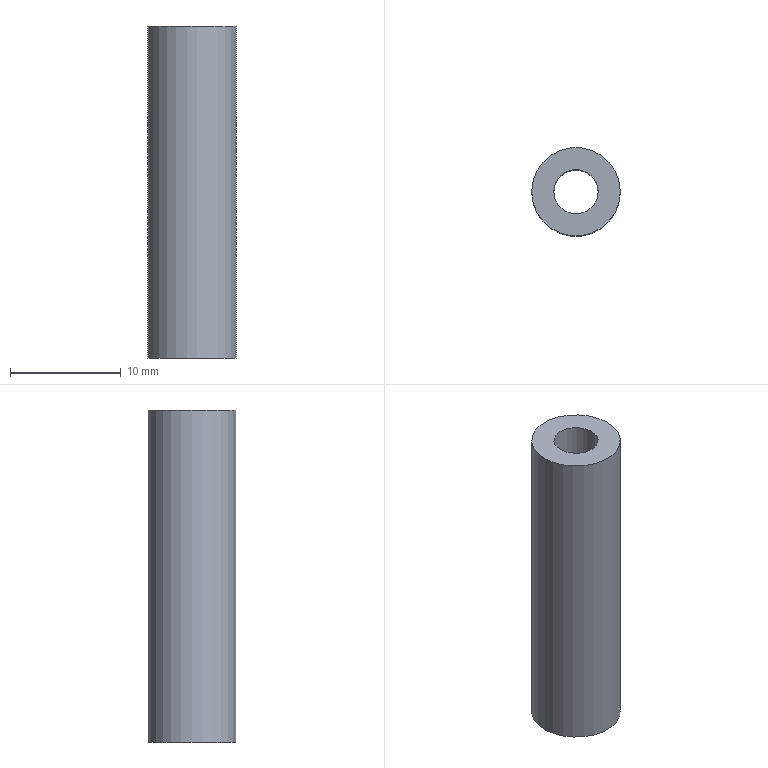Part | STEP file | gslz 2016.10.28-10_id2042_x_t | 1 solid | 4 faces | box 8 x 8 x 30 mm | volume 1131 mm3 | cylinder 2 | plane 2 | commonest cylinder face diameters 4 x1 8 x1
STEP:
#1=CARTESIAN_POINT('',(0.,0.,0.));
#2=DIRECTION('',(0.,0.,1.));
#3=DIRECTION('',(1.,0.,0.));
#4=AXIS2_PLACEMENT_3D('',#1,#2,#3);
#5=CARTESIAN_POINT('',(-541.,163.,53.));
#6=VERTEX_POINT('',#5);
#7=CARTESIAN_POINT('',(-545.,163.,53.));
#8=DIRECTION('',(0.,0.,1.));
#9=DIRECTION('',(1.,0.,0.));
#10=AXIS2_PLACEMENT_3D('',#7,#8,#9);
#11=CIRCLE('',#10,4.);
#12=CARTESIAN_POINT('',(-545.,163.,53.));
#13=DIRECTION('',(0.,0.,-1.));
#14=DIRECTION('',(1.,0.,0.));
#15=AXIS2_PLACEMENT_3D('',#12,#13,#14);
#16=CYLINDRICAL_SURFACE('',#15,4.);
#17=CARTESIAN_POINT('',(6.283,0.));
#18=DIRECTION('',(-1.,0.));
#19=VECTOR('',#18,1.);
#20=LINE('',#17,#19);
#21=(GEOMETRIC_REPRESENTATION_CONTEXT(2)PARAMETRIC_REPRESENTATION_CONTEXT()REPRESENTATION_CONTEXT('',''));
#22=DEFINITIONAL_REPRESENTATION('',(#20),#21);
#23=PCURVE('',#16,#22);
#24=CARTESIAN_POINT('',(-545.,163.,53.));
#25=DIRECTION('',(0.,0.,1.));
#26=DIRECTION('',(-1.,0.,0.));
#27=AXIS2_PLACEMENT_3D('',#24,#25,#26);
#28=PLANE('',#27);
#29=CARTESIAN_POINT('',(0.,0.));
#30=DIRECTION('',(-1.,0.));
#31=AXIS2_PLACEMENT_2D('',#29,#30);
#32=CIRCLE('',#31,4.);
#33=(GEOMETRIC_REPRESENTATION_CONTEXT(2)PARAMETRIC_REPRESENTATION_CONTEXT()REPRESENTATION_CONTEXT('',''));
#34=DEFINITIONAL_REPRESENTATION('',(#32),#33);
#35=PCURVE('',#28,#34);
#36=SURFACE_CURVE('',#11,(#23,#35),.PCURVE_S1.);
#37=EDGE_CURVE('',#6,#6,#36,.T.);
#38=ORIENTED_EDGE('',*,*,#37,.F.);
#39=CARTESIAN_POINT('',(-541.,163.,23.));
#40=VERTEX_POINT('',#39);
#41=CARTESIAN_POINT('',(-541.,163.,53.));
#42=CARTESIAN_POINT('',(-541.,163.,23.));
#43=B_SPLINE_CURVE_WITH_KNOTS('',1,(#41,#42),.UNSPECIFIED.,.F.,.F.,(2,2),(0.,30.),.PIECEWISE_BEZIER_KNOTS.);
#44=CARTESIAN_POINT('',(6.283,0.));
#45=DIRECTION('',(0.,1.));
#46=VECTOR('',#45,1.);
#47=LINE('',#44,#46);
#48=(GEOMETRIC_REPRESENTATION_CONTEXT(2)PARAMETRIC_REPRESENTATION_CONTEXT()REPRESENTATION_CONTEXT('',''));
#49=DEFINITIONAL_REPRESENTATION('',(#47),#48);
#50=PCURVE('',#16,#49);
#51=CARTESIAN_POINT('',(0.,0.));
#52=DIRECTION('',(0.,1.));
#53=VECTOR('',#52,1.);
#54=LINE('',#51,#53);
#55=(GEOMETRIC_REPRESENTATION_CONTEXT(2)PARAMETRIC_REPRESENTATION_CONTEXT()REPRESENTATION_CONTEXT('',''));
#56=DEFINITIONAL_REPRESENTATION('',(#54),#55);
#57=PCURVE('',#16,#56);
#58=SEAM_CURVE('',#43,(#50,#57),.PCURVE_S1.);
#59=EDGE_CURVE('',#6,#40,#58,.T.);
#60=ORIENTED_EDGE('',*,*,#59,.T.);
#61=CARTESIAN_POINT('',(-545.,163.,23.));
#62=DIRECTION('',(0.,0.,1.));
#63=DIRECTION('',(1.,0.,0.));
#64=AXIS2_PLACEMENT_3D('',#61,#62,#63);
#65=CIRCLE('',#64,4.);
#66=CARTESIAN_POINT('',(6.283,30.));
#67=DIRECTION('',(-1.,0.));
#68=VECTOR('',#67,1.);
#69=LINE('',#66,#68);
#70=(GEOMETRIC_REPRESENTATION_CONTEXT(2)PARAMETRIC_REPRESENTATION_CONTEXT()REPRESENTATION_CONTEXT('',''));
#71=DEFINITIONAL_REPRESENTATION('',(#69),#70);
#72=PCURVE('',#16,#71);
#73=CARTESIAN_POINT('',(-545.,163.,23.));
#74=DIRECTION('',(0.,0.,1.));
#75=DIRECTION('',(-1.,0.,0.));
#76=AXIS2_PLACEMENT_3D('',#73,#74,#75);
#77=PLANE('',#76);
#78=CARTESIAN_POINT('',(0.,0.));
#79=DIRECTION('',(-1.,0.));
#80=AXIS2_PLACEMENT_2D('',#78,#79);
#81=CIRCLE('',#80,4.);
#82=(GEOMETRIC_REPRESENTATION_CONTEXT(2)PARAMETRIC_REPRESENTATION_CONTEXT()REPRESENTATION_CONTEXT('',''));
#83=DEFINITIONAL_REPRESENTATION('',(#81),#82);
#84=PCURVE('',#77,#83);
#85=SURFACE_CURVE('',#65,(#72,#84),.PCURVE_S1.);
#86=EDGE_CURVE('',#40,#40,#85,.T.);
#87=ORIENTED_EDGE('',*,*,#86,.T.);
#88=ORIENTED_EDGE('',*,*,#59,.F.);
#89=EDGE_LOOP('',(#38,#60,#87,#88));
#90=FACE_BOUND('',#89,.T.);
#91=ADVANCED_FACE('',(#90),#16,.T.);
#92=CARTESIAN_POINT('',(-543.,163.,53.));
#93=VERTEX_POINT('',#92);
#94=CARTESIAN_POINT('',(-545.,163.,53.));
#95=DIRECTION('',(0.,0.,1.));
#96=DIRECTION('',(1.,0.,0.));
#97=AXIS2_PLACEMENT_3D('',#94,#95,#96);
#98=CIRCLE('',#97,2.);
#99=CARTESIAN_POINT('',(0.,0.));
#100=DIRECTION('',(-1.,0.));
#101=AXIS2_PLACEMENT_2D('',#99,#100);
#102=CIRCLE('',#101,2.);
#103=(GEOMETRIC_REPRESENTATION_CONTEXT(2)PARAMETRIC_REPRESENTATION_CONTEXT()REPRESENTATION_CONTEXT('',''));
#104=DEFINITIONAL_REPRESENTATION('',(#102),#103);
#105=PCURVE('',#28,#104);
#106=CARTESIAN_POINT('',(-545.,163.,-7.));
#107=DIRECTION('',(0.,0.,1.));
#108=DIRECTION('',(-1.,0.,0.));
#109=AXIS2_PLACEMENT_3D('',#106,#107,#108);
#110=CYLINDRICAL_SURFACE('',#109,2.);
#111=CARTESIAN_POINT('',(3.142,60.));
#112=DIRECTION('',(1.,0.));
#113=VECTOR('',#112,1.);
#114=LINE('',#111,#113);
#115=(GEOMETRIC_REPRESENTATION_CONTEXT(2)PARAMETRIC_REPRESENTATION_CONTEXT()REPRESENTATION_CONTEXT('',''));
#116=DEFINITIONAL_REPRESENTATION('',(#114),#115);
#117=PCURVE('',#110,#116);
#118=SURFACE_CURVE('',#98,(#105,#117),.PCURVE_S1.);
#119=EDGE_CURVE('',#93,#93,#118,.T.);
#120=ORIENTED_EDGE('',*,*,#119,.F.);
#121=EDGE_LOOP('',(#120));
#122=FACE_BOUND('',#121,.T.);
#123=ORIENTED_EDGE('',*,*,#37,.T.);
#124=EDGE_LOOP('',(#123));
#125=FACE_BOUND('',#124,.T.);
#126=ADVANCED_FACE('',(#122,#125),#28,.T.);
#127=CARTESIAN_POINT('',(-543.,163.,23.));
#128=VERTEX_POINT('',#127);
#129=CARTESIAN_POINT('',(-545.,163.,23.));
#130=DIRECTION('',(0.,0.,1.));
#131=DIRECTION('',(1.,0.,0.));
#132=AXIS2_PLACEMENT_3D('',#129,#130,#131);
#133=CIRCLE('',#132,2.);
#134=CARTESIAN_POINT('',(0.,0.));
#135=DIRECTION('',(-1.,0.));
#136=AXIS2_PLACEMENT_2D('',#134,#135);
#137=CIRCLE('',#136,2.);
#138=(GEOMETRIC_REPRESENTATION_CONTEXT(2)PARAMETRIC_REPRESENTATION_CONTEXT()REPRESENTATION_CONTEXT('',''));
#139=DEFINITIONAL_REPRESENTATION('',(#137),#138);
#140=PCURVE('',#77,#139);
#141=CARTESIAN_POINT('',(3.142,30.));
#142=DIRECTION('',(1.,0.));
#143=VECTOR('',#142,1.);
#144=LINE('',#141,#143);
#145=(GEOMETRIC_REPRESENTATION_CONTEXT(2)PARAMETRIC_REPRESENTATION_CONTEXT()REPRESENTATION_CONTEXT('',''));
#146=DEFINITIONAL_REPRESENTATION('',(#144),#145);
#147=PCURVE('',#110,#146);
#148=SURFACE_CURVE('',#133,(#140,#147),.PCURVE_S1.);
#149=EDGE_CURVE('',#128,#128,#148,.T.);
#150=ORIENTED_EDGE('',*,*,#149,.T.);
#151=EDGE_LOOP('',(#150));
#152=FACE_BOUND('',#151,.T.);
#153=ORIENTED_EDGE('',*,*,#86,.F.);
#154=EDGE_LOOP('',(#153));
#155=FACE_BOUND('',#154,.T.);
#156=ADVANCED_FACE('',(#152,#155),#77,.F.);
#157=ORIENTED_EDGE('',*,*,#119,.F.);
#158=CARTESIAN_POINT('',(-543.,163.,23.));
#159=CARTESIAN_POINT('',(-543.,163.,53.));
#160=B_SPLINE_CURVE_WITH_KNOTS('',1,(#158,#159),.UNSPECIFIED.,.F.,.F.,(2,2),(30.,60.),.PIECEWISE_BEZIER_KNOTS.);
#161=CARTESIAN_POINT('',(3.142,0.));
#162=DIRECTION('',(0.,1.));
#163=VECTOR('',#162,1.);
#164=LINE('',#161,#163);
#165=(GEOMETRIC_REPRESENTATION_CONTEXT(2)PARAMETRIC_REPRESENTATION_CONTEXT()REPRESENTATION_CONTEXT('',''));
#166=DEFINITIONAL_REPRESENTATION('',(#164),#165);
#167=PCURVE('',#110,#166);
#168=CARTESIAN_POINT('',(9.425,0.));
#169=DIRECTION('',(0.,1.));
#170=VECTOR('',#169,1.);
#171=LINE('',#168,#170);
#172=(GEOMETRIC_REPRESENTATION_CONTEXT(2)PARAMETRIC_REPRESENTATION_CONTEXT()REPRESENTATION_CONTEXT('',''));
#173=DEFINITIONAL_REPRESENTATION('',(#171),#172);
#174=PCURVE('',#110,#173);
#175=SEAM_CURVE('',#160,(#167,#174),.PCURVE_S1.);
#176=EDGE_CURVE('',#128,#93,#175,.T.);
#177=ORIENTED_EDGE('',*,*,#176,.F.);
#178=ORIENTED_EDGE('',*,*,#149,.T.);
#179=ORIENTED_EDGE('',*,*,#176,.T.);
#180=EDGE_LOOP('',(#157,#177,#178,#179));
#181=FACE_BOUND('',#180,.F.);
#182=ADVANCED_FACE('',(#181),#110,.F.);
#183=CLOSED_SHELL('',(#91,#126,#156,#182));
#184=MANIFOLD_SOLID_BREP('',#183);
#185=(LENGTH_UNIT()NAMED_UNIT(*)SI_UNIT(.MILLI.,.METRE.));
#186=UNCERTAINTY_MEASURE_WITH_UNIT(LENGTH_MEASURE(0.00001),#185,'','');
#187=(NAMED_UNIT(*)PLANE_ANGLE_UNIT()SI_UNIT($,.RADIAN.));
#188=(NAMED_UNIT(*)SI_UNIT($,.STERADIAN.)SOLID_ANGLE_UNIT());
#189=(GEOMETRIC_REPRESENTATION_CONTEXT(3)GLOBAL_UNCERTAINTY_ASSIGNED_CONTEXT((#186))GLOBAL_UNIT_ASSIGNED_CONTEXT((#185,#187,#188))REPRESENTATION_CONTEXT('',''));
#190=ADVANCED_BREP_SHAPE_REPRESENTATION('',(#4,#184),#189);